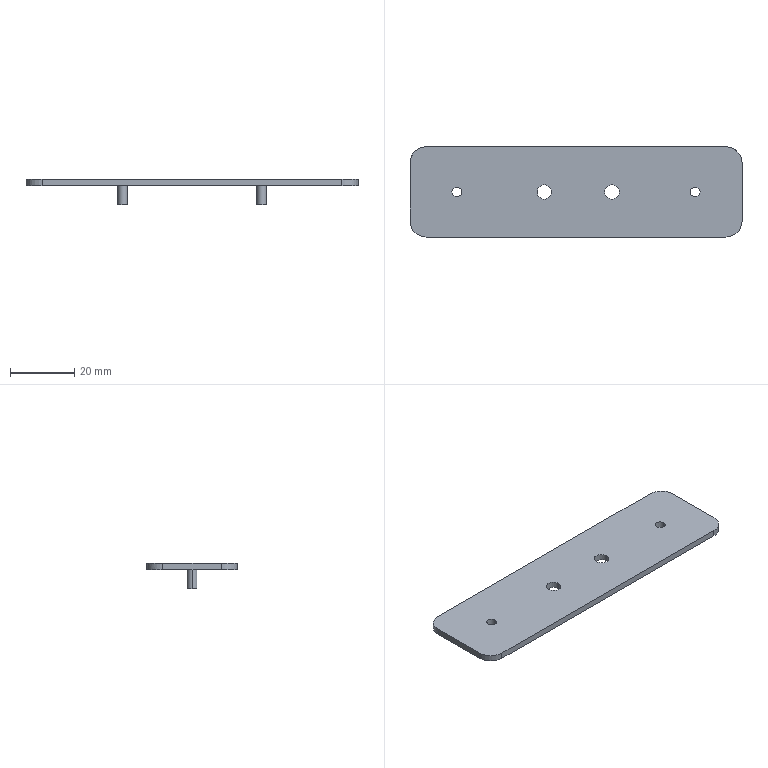Part | NX | features BREP 1 | 1 solid | 24 faces | box 103 x 28 x 8 mm | volume 5718 mm3 | cylinder 16 | plane 8 | commonest cylinder face diameters 3 x8 4.5 x4 10 x4
STEP:
#1=CARTESIAN_POINT('',(-357.75,160.5,217.465));
#2=VERTEX_POINT('',#1);
#3=CARTESIAN_POINT('',(-357.75,160.5,219.465));
#4=VERTEX_POINT('',#3);
#5=CARTESIAN_POINT('',(-357.75,160.5,217.465));
#6=DIRECTION('',(0.,0.,1.));
#7=VECTOR('',#6,1000.);
#8=LINE('',#5,#7);
#9=EDGE_CURVE('',#2,#4,#8,.T.);
#10=ORIENTED_EDGE('',*,*,#9,.T.);
#11=CARTESIAN_POINT('',(-353.25,160.5,219.465));
#12=VERTEX_POINT('',#11);
#13=CARTESIAN_POINT('',(-355.5,160.5,219.465));
#14=DIRECTION('',(0.,0.,-1.));
#15=DIRECTION('',(1.,0.,0.));
#16=AXIS2_PLACEMENT_3D('',#13,#14,#15);
#17=CIRCLE('',#16,2.25);
#18=EDGE_CURVE('',#12,#4,#17,.T.);
#19=ORIENTED_EDGE('',*,*,#18,.F.);
#20=CARTESIAN_POINT('',(-353.25,160.5,217.465));
#21=VERTEX_POINT('',#20);
#22=CARTESIAN_POINT('',(-353.25,160.5,217.465));
#23=DIRECTION('',(0.,0.,-1.));
#24=VECTOR('',#23,1000.);
#25=LINE('',#22,#24);
#26=EDGE_CURVE('',#12,#21,#25,.T.);
#27=ORIENTED_EDGE('',*,*,#26,.T.);
#28=CARTESIAN_POINT('',(-355.5,160.5,217.465));
#29=DIRECTION('',(0.,0.,1.));
#30=DIRECTION('',(1.,0.,0.));
#31=AXIS2_PLACEMENT_3D('',#28,#29,#30);
#32=CIRCLE('',#31,2.25);
#33=EDGE_CURVE('',#2,#21,#32,.T.);
#34=ORIENTED_EDGE('',*,*,#33,.F.);
#35=EDGE_LOOP('',(#10,#19,#27,#34));
#36=FACE_BOUND('',#35,.T.);
#37=CARTESIAN_POINT('',(-355.5,160.5,217.465));
#38=DIRECTION('',(0.,0.,1.));
#39=DIRECTION('',(1.,0.,0.));
#40=AXIS2_PLACEMENT_3D('',#37,#38,#39);
#41=CYLINDRICAL_SURFACE('',#40,2.25);
#42=ADVANCED_FACE('',(#36),#41,.F.);
#43=ORIENTED_EDGE('',*,*,#26,.F.);
#44=CARTESIAN_POINT('',(-355.5,160.5,219.465));
#45=DIRECTION('',(0.,0.,-1.));
#46=DIRECTION('',(1.,0.,0.));
#47=AXIS2_PLACEMENT_3D('',#44,#45,#46);
#48=CIRCLE('',#47,2.25);
#49=EDGE_CURVE('',#4,#12,#48,.T.);
#50=ORIENTED_EDGE('',*,*,#49,.F.);
#51=ORIENTED_EDGE('',*,*,#9,.F.);
#52=CARTESIAN_POINT('',(-355.5,160.5,217.465));
#53=DIRECTION('',(0.,0.,1.));
#54=DIRECTION('',(1.,0.,0.));
#55=AXIS2_PLACEMENT_3D('',#52,#53,#54);
#56=CIRCLE('',#55,2.25);
#57=EDGE_CURVE('',#21,#2,#56,.T.);
#58=ORIENTED_EDGE('',*,*,#57,.F.);
#59=EDGE_LOOP('',(#43,#50,#51,#58));
#60=FACE_BOUND('',#59,.T.);
#61=CARTESIAN_POINT('',(-355.5,160.5,217.465));
#62=DIRECTION('',(0.,0.,1.));
#63=DIRECTION('',(-1.,0.,0.));
#64=AXIS2_PLACEMENT_3D('',#61,#62,#63);
#65=CYLINDRICAL_SURFACE('',#64,2.25);
#66=ADVANCED_FACE('',(#60),#65,.F.);
#67=CARTESIAN_POINT('',(-294.175,169.5,219.465));
#68=VERTEX_POINT('',#67);
#69=CARTESIAN_POINT('',(-294.175,151.5,219.465));
#70=VERTEX_POINT('',#69);
#71=CARTESIAN_POINT('',(-294.175,160.5,219.465));
#72=DIRECTION('',(0.,-1.,0.));
#73=VECTOR('',#72,1000.);
#74=LINE('',#71,#73);
#75=EDGE_CURVE('',#68,#70,#74,.T.);
#76=ORIENTED_EDGE('',*,*,#75,.F.);
#77=CARTESIAN_POINT('',(-299.175,174.5,219.465));
#78=VERTEX_POINT('',#77);
#79=CARTESIAN_POINT('',(-299.175,174.5,219.465));
#80=CARTESIAN_POINT('',(-298.627,174.5,219.465));
#81=CARTESIAN_POINT('',(-298.08,174.425,219.465));
#82=CARTESIAN_POINT('',(-297.546,174.275,219.465));
#83=CARTESIAN_POINT('',(-296.532,173.833,219.465));
#84=CARTESIAN_POINT('',(-295.675,173.134,219.465));
#85=CARTESIAN_POINT('',(-295.297,172.728,219.465));
#86=CARTESIAN_POINT('',(-294.705,171.882,219.465));
#87=CARTESIAN_POINT('',(-294.344,170.917,219.465));
#88=CARTESIAN_POINT('',(-294.231,170.451,219.465));
#89=CARTESIAN_POINT('',(-294.175,169.975,219.465));
#90=CARTESIAN_POINT('',(-294.175,169.5,219.465));
#91=B_SPLINE_CURVE_WITH_KNOTS('',5,(#79,#80,#81,#82,#83,#84,#85,#86,#87,#88,#89,#90),.UNSPECIFIED.,.F.,.F.,(6,3,3,6),(0.,0.3487,0.6974,1.),.UNSPECIFIED.);
#92=EDGE_CURVE('',#78,#68,#91,.T.);
#93=ORIENTED_EDGE('',*,*,#92,.F.);
#94=CARTESIAN_POINT('',(-392.175,174.5,219.465));
#95=VERTEX_POINT('',#94);
#96=CARTESIAN_POINT('',(-345.675,174.5,219.465));
#97=DIRECTION('',(-1.,0.,0.));
#98=VECTOR('',#97,1000.);
#99=LINE('',#96,#98);
#100=EDGE_CURVE('',#78,#95,#99,.T.);
#101=ORIENTED_EDGE('',*,*,#100,.T.);
#102=CARTESIAN_POINT('',(-397.175,169.5,219.465));
#103=VERTEX_POINT('',#102);
#104=CARTESIAN_POINT('',(-397.175,169.5,219.465));
#105=CARTESIAN_POINT('',(-397.175,170.048,219.465));
#106=CARTESIAN_POINT('',(-397.1,170.595,219.465));
#107=CARTESIAN_POINT('',(-396.95,171.129,219.465));
#108=CARTESIAN_POINT('',(-396.508,172.143,219.465));
#109=CARTESIAN_POINT('',(-395.809,173.,219.465));
#110=CARTESIAN_POINT('',(-395.403,173.378,219.465));
#111=CARTESIAN_POINT('',(-394.557,173.97,219.465));
#112=CARTESIAN_POINT('',(-393.592,174.331,219.465));
#113=CARTESIAN_POINT('',(-393.126,174.444,219.465));
#114=CARTESIAN_POINT('',(-392.65,174.5,219.465));
#115=CARTESIAN_POINT('',(-392.175,174.5,219.465));
#116=B_SPLINE_CURVE_WITH_KNOTS('',5,(#104,#105,#106,#107,#108,#109,#110,#111,#112,#113,#114,#115),.UNSPECIFIED.,.F.,.F.,(6,3,3,6),(0.,0.3487,0.6974,1.),.UNSPECIFIED.);
#117=EDGE_CURVE('',#103,#95,#116,.T.);
#118=ORIENTED_EDGE('',*,*,#117,.F.);
#119=CARTESIAN_POINT('',(-397.175,151.5,219.465));
#120=VERTEX_POINT('',#119);
#121=CARTESIAN_POINT('',(-397.175,160.5,219.465));
#122=DIRECTION('',(0.,-1.,0.));
#123=VECTOR('',#122,1000.);
#124=LINE('',#121,#123);
#125=EDGE_CURVE('',#103,#120,#124,.T.);
#126=ORIENTED_EDGE('',*,*,#125,.T.);
#127=CARTESIAN_POINT('',(-392.175,146.5,219.465));
#128=VERTEX_POINT('',#127);
#129=CARTESIAN_POINT('',(-392.175,151.5,219.465));
#130=DIRECTION('',(0.,0.,-1.));
#131=DIRECTION('',(1.,0.,0.));
#132=AXIS2_PLACEMENT_3D('',#129,#130,#131);
#133=CIRCLE('',#132,5.);
#134=EDGE_CURVE('',#128,#120,#133,.T.);
#135=ORIENTED_EDGE('',*,*,#134,.F.);
#136=CARTESIAN_POINT('',(-299.175,146.5,219.465));
#137=VERTEX_POINT('',#136);
#138=CARTESIAN_POINT('',(-345.675,146.5,219.465));
#139=DIRECTION('',(-1.,0.,0.));
#140=VECTOR('',#139,1000.);
#141=LINE('',#138,#140);
#142=EDGE_CURVE('',#137,#128,#141,.T.);
#143=ORIENTED_EDGE('',*,*,#142,.F.);
#144=CARTESIAN_POINT('',(-299.175,151.5,219.465));
#145=DIRECTION('',(0.,0.,-1.));
#146=DIRECTION('',(1.,0.,0.));
#147=AXIS2_PLACEMENT_3D('',#144,#145,#146);
#148=CIRCLE('',#147,5.);
#149=EDGE_CURVE('',#70,#137,#148,.T.);
#150=ORIENTED_EDGE('',*,*,#149,.F.);
#151=EDGE_LOOP('',(#76,#93,#101,#118,#126,#135,#143,#150));
#152=FACE_BOUND('',#151,.T.);
#153=CARTESIAN_POINT('',(-332.25,160.5,219.465));
#154=VERTEX_POINT('',#153);
#155=CARTESIAN_POINT('',(-336.75,160.5,219.465));
#156=VERTEX_POINT('',#155);
#157=CARTESIAN_POINT('',(-334.5,160.5,219.465));
#158=DIRECTION('',(0.,0.,-1.));
#159=DIRECTION('',(1.,0.,0.));
#160=AXIS2_PLACEMENT_3D('',#157,#158,#159);
#161=CIRCLE('',#160,2.25);
#162=EDGE_CURVE('',#154,#156,#161,.T.);
#163=ORIENTED_EDGE('',*,*,#162,.T.);
#164=CARTESIAN_POINT('',(-334.5,160.5,219.465));
#165=DIRECTION('',(0.,0.,-1.));
#166=DIRECTION('',(1.,0.,0.));
#167=AXIS2_PLACEMENT_3D('',#164,#165,#166);
#168=CIRCLE('',#167,2.25);
#169=EDGE_CURVE('',#156,#154,#168,.T.);
#170=ORIENTED_EDGE('',*,*,#169,.T.);
#171=EDGE_LOOP('',(#163,#170));
#172=FACE_BOUND('',#171,.T.);
#173=CARTESIAN_POINT('',(-307.175,160.5,219.465));
#174=VERTEX_POINT('',#173);
#175=CARTESIAN_POINT('',(-310.175,160.5,219.465));
#176=VERTEX_POINT('',#175);
#177=CARTESIAN_POINT('',(-308.675,160.5,219.465));
#178=DIRECTION('',(0.,0.,-1.));
#179=DIRECTION('',(1.,0.,0.));
#180=AXIS2_PLACEMENT_3D('',#177,#178,#179);
#181=CIRCLE('',#180,1.5);
#182=EDGE_CURVE('',#174,#176,#181,.T.);
#183=ORIENTED_EDGE('',*,*,#182,.T.);
#184=CARTESIAN_POINT('',(-308.675,160.5,219.465));
#185=DIRECTION('',(0.,0.,-1.));
#186=DIRECTION('',(1.,0.,0.));
#187=AXIS2_PLACEMENT_3D('',#184,#185,#186);
#188=CIRCLE('',#187,1.5);
#189=EDGE_CURVE('',#176,#174,#188,.T.);
#190=ORIENTED_EDGE('',*,*,#189,.T.);
#191=EDGE_LOOP('',(#183,#190));
#192=FACE_BOUND('',#191,.T.);
#193=ORIENTED_EDGE('',*,*,#49,.T.);
#194=ORIENTED_EDGE('',*,*,#18,.T.);
#195=EDGE_LOOP('',(#193,#194));
#196=FACE_BOUND('',#195,.T.);
#197=CARTESIAN_POINT('',(-384.175,160.5,219.465));
#198=VERTEX_POINT('',#197);
#199=CARTESIAN_POINT('',(-381.175,160.5,219.465));
#200=VERTEX_POINT('',#199);
#201=CARTESIAN_POINT('',(-382.675,160.5,219.465));
#202=DIRECTION('',(0.,0.,-1.));
#203=DIRECTION('',(1.,0.,0.));
#204=AXIS2_PLACEMENT_3D('',#201,#202,#203);
#205=CIRCLE('',#204,1.5);
#206=EDGE_CURVE('',#198,#200,#205,.T.);
#207=ORIENTED_EDGE('',*,*,#206,.T.);
#208=CARTESIAN_POINT('',(-382.675,160.5,219.465));
#209=DIRECTION('',(0.,0.,-1.));
#210=DIRECTION('',(1.,0.,0.));
#211=AXIS2_PLACEMENT_3D('',#208,#209,#210);
#212=CIRCLE('',#211,1.5);
#213=EDGE_CURVE('',#200,#198,#212,.T.);
#214=ORIENTED_EDGE('',*,*,#213,.T.);
#215=EDGE_LOOP('',(#207,#214));
#216=FACE_BOUND('',#215,.T.);
#217=CARTESIAN_POINT('',(74.,-121.964,219.465));
#218=DIRECTION('',(0.,0.,1.));
#219=DIRECTION('',(1.,0.,0.));
#220=AXIS2_PLACEMENT_3D('',#217,#218,#219);
#221=PLANE('',#220);
#222=ADVANCED_FACE('',(#152,#172,#192,#196,#216),#221,.T.);
#223=CARTESIAN_POINT('',(-299.175,146.5,217.465));
#224=VERTEX_POINT('',#223);
#225=CARTESIAN_POINT('',(-294.175,151.5,217.465));
#226=VERTEX_POINT('',#225);
#227=CARTESIAN_POINT('',(-299.175,151.5,217.465));
#228=DIRECTION('',(0.,0.,1.));
#229=DIRECTION('',(1.,0.,0.));
#230=AXIS2_PLACEMENT_3D('',#227,#228,#229);
#231=CIRCLE('',#230,5.);
#232=EDGE_CURVE('',#224,#226,#231,.T.);
#233=ORIENTED_EDGE('',*,*,#232,.F.);
#234=CARTESIAN_POINT('',(-392.175,146.5,217.465));
#235=VERTEX_POINT('',#234);
#236=CARTESIAN_POINT('',(-345.675,146.5,217.465));
#237=DIRECTION('',(-1.,0.,0.));
#238=VECTOR('',#237,1000.);
#239=LINE('',#236,#238);
#240=EDGE_CURVE('',#224,#235,#239,.T.);
#241=ORIENTED_EDGE('',*,*,#240,.T.);
#242=CARTESIAN_POINT('',(-397.175,151.5,217.465));
#243=VERTEX_POINT('',#242);
#244=CARTESIAN_POINT('',(-392.175,151.5,217.465));
#245=DIRECTION('',(0.,0.,1.));
#246=DIRECTION('',(1.,0.,0.));
#247=AXIS2_PLACEMENT_3D('',#244,#245,#246);
#248=CIRCLE('',#247,5.);
#249=EDGE_CURVE('',#243,#235,#248,.T.);
#250=ORIENTED_EDGE('',*,*,#249,.F.);
#251=CARTESIAN_POINT('',(-397.175,169.5,217.465));
#252=VERTEX_POINT('',#251);
#253=CARTESIAN_POINT('',(-397.175,160.5,217.465));
#254=DIRECTION('',(0.,-1.,0.));
#255=VECTOR('',#254,1000.);
#256=LINE('',#253,#255);
#257=EDGE_CURVE('',#252,#243,#256,.T.);
#258=ORIENTED_EDGE('',*,*,#257,.F.);
#259=CARTESIAN_POINT('',(-392.175,174.5,217.465));
#260=VERTEX_POINT('',#259);
#261=CARTESIAN_POINT('',(-392.175,174.5,217.465));
#262=CARTESIAN_POINT('',(-392.65,174.5,217.465));
#263=CARTESIAN_POINT('',(-393.126,174.444,217.465));
#264=CARTESIAN_POINT('',(-393.592,174.331,217.465));
#265=CARTESIAN_POINT('',(-394.557,173.97,217.465));
#266=CARTESIAN_POINT('',(-395.403,173.378,217.465));
#267=CARTESIAN_POINT('',(-395.809,173.,217.465));
#268=CARTESIAN_POINT('',(-396.508,172.143,217.465));
#269=CARTESIAN_POINT('',(-396.95,171.129,217.465));
#270=CARTESIAN_POINT('',(-397.1,170.595,217.465));
#271=CARTESIAN_POINT('',(-397.175,170.048,217.465));
#272=CARTESIAN_POINT('',(-397.175,169.5,217.465));
#273=B_SPLINE_CURVE_WITH_KNOTS('',5,(#261,#262,#263,#264,#265,#266,#267,#268,#269,#270,#271,#272),.UNSPECIFIED.,.F.,.F.,(6,3,3,6),(0.,0.3026,0.6513,1.),.UNSPECIFIED.);
#274=EDGE_CURVE('',#260,#252,#273,.T.);
#275=ORIENTED_EDGE('',*,*,#274,.F.);
#276=CARTESIAN_POINT('',(-299.175,174.5,217.465));
#277=VERTEX_POINT('',#276);
#278=CARTESIAN_POINT('',(-345.675,174.5,217.465));
#279=DIRECTION('',(-1.,0.,0.));
#280=VECTOR('',#279,1000.);
#281=LINE('',#278,#280);
#282=EDGE_CURVE('',#277,#260,#281,.T.);
#283=ORIENTED_EDGE('',*,*,#282,.F.);
#284=CARTESIAN_POINT('',(-294.175,169.5,217.465));
#285=VERTEX_POINT('',#284);
#286=CARTESIAN_POINT('',(-294.175,169.5,217.465));
#287=CARTESIAN_POINT('',(-294.175,169.975,217.465));
#288=CARTESIAN_POINT('',(-294.231,170.451,217.465));
#289=CARTESIAN_POINT('',(-294.344,170.917,217.465));
#290=CARTESIAN_POINT('',(-294.705,171.882,217.465));
#291=CARTESIAN_POINT('',(-295.297,172.728,217.465));
#292=CARTESIAN_POINT('',(-295.675,173.134,217.465));
#293=CARTESIAN_POINT('',(-296.532,173.833,217.465));
#294=CARTESIAN_POINT('',(-297.546,174.275,217.465));
#295=CARTESIAN_POINT('',(-298.08,174.425,217.465));
#296=CARTESIAN_POINT('',(-298.627,174.5,217.465));
#297=CARTESIAN_POINT('',(-299.175,174.5,217.465));
#298=B_SPLINE_CURVE_WITH_KNOTS('',5,(#286,#287,#288,#289,#290,#291,#292,#293,#294,#295,#296,#297),.UNSPECIFIED.,.F.,.F.,(6,3,3,6),(0.,0.3026,0.6513,1.),.UNSPECIFIED.);
#299=EDGE_CURVE('',#285,#277,#298,.T.);
#300=ORIENTED_EDGE('',*,*,#299,.F.);
#301=CARTESIAN_POINT('',(-294.175,160.5,217.465));
#302=DIRECTION('',(0.,-1.,0.));
#303=VECTOR('',#302,1000.);
#304=LINE('',#301,#303);
#305=EDGE_CURVE('',#285,#226,#304,.T.);
#306=ORIENTED_EDGE('',*,*,#305,.T.);
#307=EDGE_LOOP('',(#233,#241,#250,#258,#275,#283,#300,#306));
#308=FACE_BOUND('',#307,.T.);
#309=CARTESIAN_POINT('',(-322.675,160.5,217.465));
#310=VERTEX_POINT('',#309);
#311=CARTESIAN_POINT('',(-325.675,160.5,217.465));
#312=VERTEX_POINT('',#311);
#313=CARTESIAN_POINT('',(-324.175,160.5,217.465));
#314=DIRECTION('',(0.,0.,1.));
#315=DIRECTION('',(1.,0.,0.));
#316=AXIS2_PLACEMENT_3D('',#313,#314,#315);
#317=CIRCLE('',#316,1.5);
#318=EDGE_CURVE('',#310,#312,#317,.T.);
#319=ORIENTED_EDGE('',*,*,#318,.T.);
#320=CARTESIAN_POINT('',(-324.175,160.5,217.465));
#321=DIRECTION('',(0.,0.,1.));
#322=DIRECTION('',(1.,0.,0.));
#323=AXIS2_PLACEMENT_3D('',#320,#321,#322);
#324=CIRCLE('',#323,1.5);
#325=EDGE_CURVE('',#312,#310,#324,.T.);
#326=ORIENTED_EDGE('',*,*,#325,.T.);
#327=EDGE_LOOP('',(#319,#326));
#328=FACE_BOUND('',#327,.T.);
#329=CARTESIAN_POINT('',(-365.675,160.5,217.465));
#330=VERTEX_POINT('',#329);
#331=CARTESIAN_POINT('',(-368.675,160.5,217.465));
#332=VERTEX_POINT('',#331);
#333=CARTESIAN_POINT('',(-367.175,160.5,217.465));
#334=DIRECTION('',(0.,0.,1.));
#335=DIRECTION('',(1.,0.,0.));
#336=AXIS2_PLACEMENT_3D('',#333,#334,#335);
#337=CIRCLE('',#336,1.5);
#338=EDGE_CURVE('',#330,#332,#337,.T.);
#339=ORIENTED_EDGE('',*,*,#338,.T.);
#340=CARTESIAN_POINT('',(-367.175,160.5,217.465));
#341=DIRECTION('',(0.,0.,1.));
#342=DIRECTION('',(1.,0.,0.));
#343=AXIS2_PLACEMENT_3D('',#340,#341,#342);
#344=CIRCLE('',#343,1.5);
#345=EDGE_CURVE('',#332,#330,#344,.T.);
#346=ORIENTED_EDGE('',*,*,#345,.T.);
#347=EDGE_LOOP('',(#339,#346));
#348=FACE_BOUND('',#347,.T.);
#349=ORIENTED_EDGE('',*,*,#57,.T.);
#350=ORIENTED_EDGE('',*,*,#33,.T.);
#351=EDGE_LOOP('',(#349,#350));
#352=FACE_BOUND('',#351,.T.);
#353=CARTESIAN_POINT('',(-332.25,160.5,217.465));
#354=VERTEX_POINT('',#353);
#355=CARTESIAN_POINT('',(-336.75,160.5,217.465));
#356=VERTEX_POINT('',#355);
#357=CARTESIAN_POINT('',(-334.5,160.5,217.465));
#358=DIRECTION('',(0.,0.,1.));
#359=DIRECTION('',(1.,0.,0.));
#360=AXIS2_PLACEMENT_3D('',#357,#358,#359);
#361=CIRCLE('',#360,2.25);
#362=EDGE_CURVE('',#354,#356,#361,.T.);
#363=ORIENTED_EDGE('',*,*,#362,.T.);
#364=CARTESIAN_POINT('',(-334.5,160.5,217.465));
#365=DIRECTION('',(0.,0.,1.));
#366=DIRECTION('',(1.,0.,0.));
#367=AXIS2_PLACEMENT_3D('',#364,#365,#366);
#368=CIRCLE('',#367,2.25);
#369=EDGE_CURVE('',#356,#354,#368,.T.);
#370=ORIENTED_EDGE('',*,*,#369,.T.);
#371=EDGE_LOOP('',(#363,#370));
#372=FACE_BOUND('',#371,.T.);
#373=CARTESIAN_POINT('',(-381.175,160.5,217.465));
#374=VERTEX_POINT('',#373);
#375=CARTESIAN_POINT('',(-384.175,160.5,217.465));
#376=VERTEX_POINT('',#375);
#377=CARTESIAN_POINT('',(-382.675,160.5,217.465));
#378=DIRECTION('',(0.,0.,1.));
#379=DIRECTION('',(1.,0.,0.));
#380=AXIS2_PLACEMENT_3D('',#377,#378,#379);
#381=CIRCLE('',#380,1.5);
#382=EDGE_CURVE('',#374,#376,#381,.T.);
#383=ORIENTED_EDGE('',*,*,#382,.T.);
#384=CARTESIAN_POINT('',(-382.675,160.5,217.465));
#385=DIRECTION('',(0.,0.,1.));
#386=DIRECTION('',(1.,0.,0.));
#387=AXIS2_PLACEMENT_3D('',#384,#385,#386);
#388=CIRCLE('',#387,1.5);
#389=EDGE_CURVE('',#376,#374,#388,.T.);
#390=ORIENTED_EDGE('',*,*,#389,.T.);
#391=EDGE_LOOP('',(#383,#390));
#392=FACE_BOUND('',#391,.T.);
#393=CARTESIAN_POINT('',(-307.175,160.5,217.465));
#394=VERTEX_POINT('',#393);
#395=CARTESIAN_POINT('',(-310.175,160.5,217.465));
#396=VERTEX_POINT('',#395);
#397=CARTESIAN_POINT('',(-308.675,160.5,217.465));
#398=DIRECTION('',(0.,0.,1.));
#399=DIRECTION('',(1.,0.,0.));
#400=AXIS2_PLACEMENT_3D('',#397,#398,#399);
#401=CIRCLE('',#400,1.5);
#402=EDGE_CURVE('',#394,#396,#401,.T.);
#403=ORIENTED_EDGE('',*,*,#402,.T.);
#404=CARTESIAN_POINT('',(-308.675,160.5,217.465));
#405=DIRECTION('',(0.,0.,1.));
#406=DIRECTION('',(1.,0.,0.));
#407=AXIS2_PLACEMENT_3D('',#404,#405,#406);
#408=CIRCLE('',#407,1.5);
#409=EDGE_CURVE('',#396,#394,#408,.T.);
#410=ORIENTED_EDGE('',*,*,#409,.T.);
#411=EDGE_LOOP('',(#403,#410));
#412=FACE_BOUND('',#411,.T.);
#413=CARTESIAN_POINT('',(74.,-121.964,217.465));
#414=DIRECTION('',(0.,0.,1.));
#415=DIRECTION('',(1.,0.,0.));
#416=AXIS2_PLACEMENT_3D('',#413,#414,#415);
#417=PLANE('',#416);
#418=ADVANCED_FACE('',(#308,#328,#348,#352,#372,#392,#412),#417,.F.);
#419=ORIENTED_EDGE('',*,*,#305,.F.);
#420=CARTESIAN_POINT('',(-294.175,169.5,218.465));
#421=DIRECTION('',(0.,-0.000000001,-1.));
#422=VECTOR('',#421,1000.);
#423=LINE('',#420,#422);
#424=EDGE_CURVE('',#68,#285,#423,.T.);
#425=ORIENTED_EDGE('',*,*,#424,.F.);
#426=ORIENTED_EDGE('',*,*,#75,.T.);
#427=CARTESIAN_POINT('',(-294.175,151.5,218.465));
#428=DIRECTION('',(0.,0.,1.));
#429=VECTOR('',#428,1000.);
#430=LINE('',#427,#429);
#431=EDGE_CURVE('',#226,#70,#430,.T.);
#432=ORIENTED_EDGE('',*,*,#431,.F.);
#433=EDGE_LOOP('',(#419,#425,#426,#432));
#434=FACE_BOUND('',#433,.T.);
#435=CARTESIAN_POINT('',(-294.175,146.5,217.465));
#436=DIRECTION('',(1.,0.,0.));
#437=DIRECTION('',(0.,1.,0.));
#438=AXIS2_PLACEMENT_3D('',#435,#436,#437);
#439=PLANE('',#438);
#440=ADVANCED_FACE('',(#434),#439,.T.);
#441=ORIENTED_EDGE('',*,*,#299,.T.);
#442=CARTESIAN_POINT('',(-299.175,174.5,218.465));
#443=DIRECTION('',(0.,0.,-1.));
#444=VECTOR('',#443,1000.);
#445=LINE('',#442,#444);
#446=EDGE_CURVE('',#78,#277,#445,.T.);
#447=ORIENTED_EDGE('',*,*,#446,.F.);
#448=ORIENTED_EDGE('',*,*,#92,.T.);
#449=ORIENTED_EDGE('',*,*,#424,.T.);
#450=EDGE_LOOP('',(#441,#447,#448,#449));
#451=FACE_BOUND('',#450,.T.);
#452=CARTESIAN_POINT('',(-299.175,169.5,218.465));
#453=DIRECTION('',(0.,0.,-1.));
#454=DIRECTION('',(0.,-1.,0.));
#455=AXIS2_PLACEMENT_3D('',#452,#453,#454);
#456=CYLINDRICAL_SURFACE('',#455,5.);
#457=ADVANCED_FACE('',(#451),#456,.T.);
#458=ORIENTED_EDGE('',*,*,#282,.T.);
#459=CARTESIAN_POINT('',(-392.175,174.5,218.465));
#460=DIRECTION('',(0.,0.,-1.));
#461=VECTOR('',#460,1000.);
#462=LINE('',#459,#461);
#463=EDGE_CURVE('',#95,#260,#462,.T.);
#464=ORIENTED_EDGE('',*,*,#463,.F.);
#465=ORIENTED_EDGE('',*,*,#100,.F.);
#466=ORIENTED_EDGE('',*,*,#446,.T.);
#467=EDGE_LOOP('',(#458,#464,#465,#466));
#468=FACE_BOUND('',#467,.T.);
#469=CARTESIAN_POINT('',(-294.125,174.5,217.465));
#470=DIRECTION('',(0.,1.,0.));
#471=DIRECTION('',(1.,0.,0.));
#472=AXIS2_PLACEMENT_3D('',#469,#470,#471);
#473=PLANE('',#472);
#474=ADVANCED_FACE('',(#468),#473,.T.);
#475=ORIENTED_EDGE('',*,*,#274,.T.);
#476=CARTESIAN_POINT('',(-397.175,169.5,218.465));
#477=DIRECTION('',(0.,0.,-1.));
#478=VECTOR('',#477,1000.);
#479=LINE('',#476,#478);
#480=EDGE_CURVE('',#103,#252,#479,.T.);
#481=ORIENTED_EDGE('',*,*,#480,.F.);
#482=ORIENTED_EDGE('',*,*,#117,.T.);
#483=ORIENTED_EDGE('',*,*,#463,.T.);
#484=EDGE_LOOP('',(#475,#481,#482,#483));
#485=FACE_BOUND('',#484,.T.);
#486=CARTESIAN_POINT('',(-392.175,169.5,218.465));
#487=DIRECTION('',(0.,0.,-1.));
#488=DIRECTION('',(1.,0.,0.));
#489=AXIS2_PLACEMENT_3D('',#486,#487,#488);
#490=CYLINDRICAL_SURFACE('',#489,5.);
#491=ADVANCED_FACE('',(#485),#490,.T.);
#492=ORIENTED_EDGE('',*,*,#125,.F.);
#493=ORIENTED_EDGE('',*,*,#480,.T.);
#494=ORIENTED_EDGE('',*,*,#257,.T.);
#495=CARTESIAN_POINT('',(-397.175,151.5,218.465));
#496=DIRECTION('',(0.,0.,1.));
#497=VECTOR('',#496,1000.);
#498=LINE('',#495,#497);
#499=EDGE_CURVE('',#243,#120,#498,.T.);
#500=ORIENTED_EDGE('',*,*,#499,.T.);
#501=EDGE_LOOP('',(#492,#493,#494,#500));
#502=FACE_BOUND('',#501,.T.);
#503=CARTESIAN_POINT('',(-397.175,174.5,217.465));
#504=DIRECTION('',(-1.,0.,0.));
#505=DIRECTION('',(0.,0.,1.));
#506=AXIS2_PLACEMENT_3D('',#503,#504,#505);
#507=PLANE('',#506);
#508=ADVANCED_FACE('',(#502),#507,.T.);
#509=ORIENTED_EDGE('',*,*,#134,.T.);
#510=ORIENTED_EDGE('',*,*,#499,.F.);
#511=ORIENTED_EDGE('',*,*,#249,.T.);
#512=CARTESIAN_POINT('',(-392.175,146.5,218.465));
#513=DIRECTION('',(0.,0.,1.));
#514=VECTOR('',#513,1000.);
#515=LINE('',#512,#514);
#516=EDGE_CURVE('',#235,#128,#515,.T.);
#517=ORIENTED_EDGE('',*,*,#516,.T.);
#518=EDGE_LOOP('',(#509,#510,#511,#517));
#519=FACE_BOUND('',#518,.T.);
#520=CARTESIAN_POINT('',(-392.175,151.5,218.465));
#521=DIRECTION('',(0.,0.,1.));
#522=DIRECTION('',(1.,0.,0.));
#523=AXIS2_PLACEMENT_3D('',#520,#521,#522);
#524=CYLINDRICAL_SURFACE('',#523,5.);
#525=ADVANCED_FACE('',(#519),#524,.T.);
#526=ORIENTED_EDGE('',*,*,#142,.T.);
#527=ORIENTED_EDGE('',*,*,#516,.F.);
#528=ORIENTED_EDGE('',*,*,#240,.F.);
#529=CARTESIAN_POINT('',(-299.175,146.5,218.465));
#530=DIRECTION('',(0.,0.,1.));
#531=VECTOR('',#530,1000.);
#532=LINE('',#529,#531);
#533=EDGE_CURVE('',#224,#137,#532,.T.);
#534=ORIENTED_EDGE('',*,*,#533,.T.);
#535=EDGE_LOOP('',(#526,#527,#528,#534));
#536=FACE_BOUND('',#535,.T.);
#537=CARTESIAN_POINT('',(-397.225,146.5,217.465));
#538=DIRECTION('',(0.,-1.,0.));
#539=DIRECTION('',(0.,0.,-1.));
#540=AXIS2_PLACEMENT_3D('',#537,#538,#539);
#541=PLANE('',#540);
#542=ADVANCED_FACE('',(#536),#541,.T.);
#543=ORIENTED_EDGE('',*,*,#149,.T.);
#544=ORIENTED_EDGE('',*,*,#533,.F.);
#545=ORIENTED_EDGE('',*,*,#232,.T.);
#546=ORIENTED_EDGE('',*,*,#431,.T.);
#547=EDGE_LOOP('',(#543,#544,#545,#546));
#548=FACE_BOUND('',#547,.T.);
#549=CARTESIAN_POINT('',(-299.175,151.5,218.465));
#550=DIRECTION('',(0.,0.,1.));
#551=DIRECTION('',(0.,1.,0.));
#552=AXIS2_PLACEMENT_3D('',#549,#550,#551);
#553=CYLINDRICAL_SURFACE('',#552,5.);
#554=ADVANCED_FACE('',(#548),#553,.T.);
#555=CARTESIAN_POINT('',(-336.75,160.5,217.465));
#556=DIRECTION('',(0.,0.,1.));
#557=VECTOR('',#556,1000.);
#558=LINE('',#555,#557);
#559=EDGE_CURVE('',#356,#156,#558,.T.);
#560=ORIENTED_EDGE('',*,*,#559,.T.);
#561=ORIENTED_EDGE('',*,*,#162,.F.);
#562=CARTESIAN_POINT('',(-332.25,160.5,217.465));
#563=DIRECTION('',(0.,0.,-1.));
#564=VECTOR('',#563,1000.);
#565=LINE('',#562,#564);
#566=EDGE_CURVE('',#154,#354,#565,.T.);
#567=ORIENTED_EDGE('',*,*,#566,.T.);
#568=ORIENTED_EDGE('',*,*,#369,.F.);
#569=EDGE_LOOP('',(#560,#561,#567,#568));
#570=FACE_BOUND('',#569,.T.);
#571=CARTESIAN_POINT('',(-334.5,160.5,217.465));
#572=DIRECTION('',(0.,0.,1.));
#573=DIRECTION('',(1.,0.,0.));
#574=AXIS2_PLACEMENT_3D('',#571,#572,#573);
#575=CYLINDRICAL_SURFACE('',#574,2.25);
#576=ADVANCED_FACE('',(#570),#575,.F.);
#577=ORIENTED_EDGE('',*,*,#566,.F.);
#578=ORIENTED_EDGE('',*,*,#169,.F.);
#579=ORIENTED_EDGE('',*,*,#559,.F.);
#580=ORIENTED_EDGE('',*,*,#362,.F.);
#581=EDGE_LOOP('',(#577,#578,#579,#580));
#582=FACE_BOUND('',#581,.T.);
#583=CARTESIAN_POINT('',(-334.5,160.5,217.465));
#584=DIRECTION('',(0.,0.,1.));
#585=DIRECTION('',(-1.,0.,0.));
#586=AXIS2_PLACEMENT_3D('',#583,#584,#585);
#587=CYLINDRICAL_SURFACE('',#586,2.25);
#588=ADVANCED_FACE('',(#582),#587,.F.);
#589=CARTESIAN_POINT('',(-310.175,160.5,217.465));
#590=DIRECTION('',(0.,0.,1.));
#591=VECTOR('',#590,1000.);
#592=LINE('',#589,#591);
#593=EDGE_CURVE('',#396,#176,#592,.T.);
#594=ORIENTED_EDGE('',*,*,#593,.T.);
#595=ORIENTED_EDGE('',*,*,#182,.F.);
#596=CARTESIAN_POINT('',(-307.175,160.5,217.465));
#597=DIRECTION('',(0.,0.,-1.));
#598=VECTOR('',#597,1000.);
#599=LINE('',#596,#598);
#600=EDGE_CURVE('',#174,#394,#599,.T.);
#601=ORIENTED_EDGE('',*,*,#600,.T.);
#602=ORIENTED_EDGE('',*,*,#409,.F.);
#603=EDGE_LOOP('',(#594,#595,#601,#602));
#604=FACE_BOUND('',#603,.T.);
#605=CARTESIAN_POINT('',(-308.675,160.5,217.465));
#606=DIRECTION('',(0.,0.,1.));
#607=DIRECTION('',(1.,0.,0.));
#608=AXIS2_PLACEMENT_3D('',#605,#606,#607);
#609=CYLINDRICAL_SURFACE('',#608,1.5);
#610=ADVANCED_FACE('',(#604),#609,.F.);
#611=ORIENTED_EDGE('',*,*,#600,.F.);
#612=ORIENTED_EDGE('',*,*,#189,.F.);
#613=ORIENTED_EDGE('',*,*,#593,.F.);
#614=ORIENTED_EDGE('',*,*,#402,.F.);
#615=EDGE_LOOP('',(#611,#612,#613,#614));
#616=FACE_BOUND('',#615,.T.);
#617=CARTESIAN_POINT('',(-308.675,160.5,217.465));
#618=DIRECTION('',(0.,0.,1.));
#619=DIRECTION('',(-1.,0.,0.));
#620=AXIS2_PLACEMENT_3D('',#617,#618,#619);
#621=CYLINDRICAL_SURFACE('',#620,1.5);
#622=ADVANCED_FACE('',(#616),#621,.F.);
#623=CARTESIAN_POINT('',(-381.175,160.5,217.465));
#624=DIRECTION('',(0.,0.,-1.));
#625=VECTOR('',#624,1000.);
#626=LINE('',#623,#625);
#627=EDGE_CURVE('',#200,#374,#626,.T.);
#628=ORIENTED_EDGE('',*,*,#627,.F.);
#629=ORIENTED_EDGE('',*,*,#206,.F.);
#630=CARTESIAN_POINT('',(-384.175,160.5,217.465));
#631=DIRECTION('',(0.,0.,1.));
#632=VECTOR('',#631,1000.);
#633=LINE('',#630,#632);
#634=EDGE_CURVE('',#376,#198,#633,.T.);
#635=ORIENTED_EDGE('',*,*,#634,.F.);
#636=ORIENTED_EDGE('',*,*,#382,.F.);
#637=EDGE_LOOP('',(#628,#629,#635,#636));
#638=FACE_BOUND('',#637,.T.);
#639=CARTESIAN_POINT('',(-382.675,160.5,217.465));
#640=DIRECTION('',(0.,0.,1.));
#641=DIRECTION('',(-1.,0.,0.));
#642=AXIS2_PLACEMENT_3D('',#639,#640,#641);
#643=CYLINDRICAL_SURFACE('',#642,1.5);
#644=ADVANCED_FACE('',(#638),#643,.F.);
#645=ORIENTED_EDGE('',*,*,#634,.T.);
#646=ORIENTED_EDGE('',*,*,#213,.F.);
#647=ORIENTED_EDGE('',*,*,#627,.T.);
#648=ORIENTED_EDGE('',*,*,#389,.F.);
#649=EDGE_LOOP('',(#645,#646,#647,#648));
#650=FACE_BOUND('',#649,.T.);
#651=CARTESIAN_POINT('',(-382.675,160.5,217.465));
#652=DIRECTION('',(0.,0.,1.));
#653=DIRECTION('',(1.,0.,0.));
#654=AXIS2_PLACEMENT_3D('',#651,#652,#653);
#655=CYLINDRICAL_SURFACE('',#654,1.5);
#656=ADVANCED_FACE('',(#650),#655,.F.);
#657=CARTESIAN_POINT('',(-322.675,160.5,211.465));
#658=VERTEX_POINT('',#657);
#659=CARTESIAN_POINT('',(-325.675,160.5,211.465));
#660=VERTEX_POINT('',#659);
#661=CARTESIAN_POINT('',(-324.175,160.5,211.465));
#662=DIRECTION('',(0.,0.,1.));
#663=DIRECTION('',(1.,0.,0.));
#664=AXIS2_PLACEMENT_3D('',#661,#662,#663);
#665=CIRCLE('',#664,1.5);
#666=EDGE_CURVE('',#658,#660,#665,.T.);
#667=ORIENTED_EDGE('',*,*,#666,.F.);
#668=CARTESIAN_POINT('',(-324.175,160.5,211.465));
#669=DIRECTION('',(0.,0.,1.));
#670=DIRECTION('',(1.,0.,0.));
#671=AXIS2_PLACEMENT_3D('',#668,#669,#670);
#672=CIRCLE('',#671,1.5);
#673=EDGE_CURVE('',#660,#658,#672,.T.);
#674=ORIENTED_EDGE('',*,*,#673,.F.);
#675=EDGE_LOOP('',(#667,#674));
#676=FACE_BOUND('',#675,.T.);
#677=CARTESIAN_POINT('',(0.,0.,211.465));
#678=DIRECTION('',(0.,0.,1.));
#679=DIRECTION('',(-1.,0.,0.));
#680=AXIS2_PLACEMENT_3D('',#677,#678,#679);
#681=PLANE('',#680);
#682=ADVANCED_FACE('',(#676),#681,.F.);
#683=CARTESIAN_POINT('',(-365.675,160.5,211.465));
#684=VERTEX_POINT('',#683);
#685=CARTESIAN_POINT('',(-368.675,160.5,211.465));
#686=VERTEX_POINT('',#685);
#687=CARTESIAN_POINT('',(-367.175,160.5,211.465));
#688=DIRECTION('',(0.,0.,1.));
#689=DIRECTION('',(1.,0.,0.));
#690=AXIS2_PLACEMENT_3D('',#687,#688,#689);
#691=CIRCLE('',#690,1.5);
#692=EDGE_CURVE('',#684,#686,#691,.T.);
#693=ORIENTED_EDGE('',*,*,#692,.F.);
#694=CARTESIAN_POINT('',(-367.175,160.5,211.465));
#695=DIRECTION('',(0.,0.,1.));
#696=DIRECTION('',(1.,0.,0.));
#697=AXIS2_PLACEMENT_3D('',#694,#695,#696);
#698=CIRCLE('',#697,1.5);
#699=EDGE_CURVE('',#686,#684,#698,.T.);
#700=ORIENTED_EDGE('',*,*,#699,.F.);
#701=EDGE_LOOP('',(#693,#700));
#702=FACE_BOUND('',#701,.T.);
#703=CARTESIAN_POINT('',(0.,0.,211.465));
#704=DIRECTION('',(0.,0.,1.));
#705=DIRECTION('',(-1.,0.,0.));
#706=AXIS2_PLACEMENT_3D('',#703,#704,#705);
#707=PLANE('',#706);
#708=ADVANCED_FACE('',(#702),#707,.F.);
#709=CARTESIAN_POINT('',(-365.675,160.5,216.465));
#710=DIRECTION('',(0.,0.,-1.));
#711=VECTOR('',#710,1000.);
#712=LINE('',#709,#711);
#713=EDGE_CURVE('',#330,#684,#712,.T.);
#714=ORIENTED_EDGE('',*,*,#713,.F.);
#715=ORIENTED_EDGE('',*,*,#345,.F.);
#716=CARTESIAN_POINT('',(-368.675,160.5,216.465));
#717=DIRECTION('',(0.,0.,-1.));
#718=VECTOR('',#717,1000.);
#719=LINE('',#716,#718);
#720=EDGE_CURVE('',#332,#686,#719,.T.);
#721=ORIENTED_EDGE('',*,*,#720,.T.);
#722=ORIENTED_EDGE('',*,*,#699,.T.);
#723=EDGE_LOOP('',(#714,#715,#721,#722));
#724=FACE_BOUND('',#723,.T.);
#725=CARTESIAN_POINT('',(-367.175,160.5,216.465));
#726=DIRECTION('',(0.,0.,1.));
#727=DIRECTION('',(1.,0.,0.));
#728=AXIS2_PLACEMENT_3D('',#725,#726,#727);
#729=CYLINDRICAL_SURFACE('',#728,1.5);
#730=ADVANCED_FACE('',(#724),#729,.T.);
#731=ORIENTED_EDGE('',*,*,#713,.T.);
#732=ORIENTED_EDGE('',*,*,#692,.T.);
#733=ORIENTED_EDGE('',*,*,#720,.F.);
#734=ORIENTED_EDGE('',*,*,#338,.F.);
#735=EDGE_LOOP('',(#731,#732,#733,#734));
#736=FACE_BOUND('',#735,.T.);
#737=CARTESIAN_POINT('',(-367.175,160.5,216.465));
#738=DIRECTION('',(0.,0.,1.));
#739=DIRECTION('',(-1.,0.,0.));
#740=AXIS2_PLACEMENT_3D('',#737,#738,#739);
#741=CYLINDRICAL_SURFACE('',#740,1.5);
#742=ADVANCED_FACE('',(#736),#741,.T.);
#743=CARTESIAN_POINT('',(-322.675,160.5,216.465));
#744=DIRECTION('',(0.,0.,-1.));
#745=VECTOR('',#744,1000.);
#746=LINE('',#743,#745);
#747=EDGE_CURVE('',#310,#658,#746,.T.);
#748=ORIENTED_EDGE('',*,*,#747,.F.);
#749=ORIENTED_EDGE('',*,*,#325,.F.);
#750=CARTESIAN_POINT('',(-325.675,160.5,216.465));
#751=DIRECTION('',(0.,0.,-1.));
#752=VECTOR('',#751,1000.);
#753=LINE('',#750,#752);
#754=EDGE_CURVE('',#312,#660,#753,.T.);
#755=ORIENTED_EDGE('',*,*,#754,.T.);
#756=ORIENTED_EDGE('',*,*,#673,.T.);
#757=EDGE_LOOP('',(#748,#749,#755,#756));
#758=FACE_BOUND('',#757,.T.);
#759=CARTESIAN_POINT('',(-324.175,160.5,216.465));
#760=DIRECTION('',(0.,0.,1.));
#761=DIRECTION('',(1.,0.,0.));
#762=AXIS2_PLACEMENT_3D('',#759,#760,#761);
#763=CYLINDRICAL_SURFACE('',#762,1.5);
#764=ADVANCED_FACE('',(#758),#763,.T.);
#765=ORIENTED_EDGE('',*,*,#747,.T.);
#766=ORIENTED_EDGE('',*,*,#666,.T.);
#767=ORIENTED_EDGE('',*,*,#754,.F.);
#768=ORIENTED_EDGE('',*,*,#318,.F.);
#769=EDGE_LOOP('',(#765,#766,#767,#768));
#770=FACE_BOUND('',#769,.T.);
#771=CARTESIAN_POINT('',(-324.175,160.5,216.465));
#772=DIRECTION('',(0.,0.,1.));
#773=DIRECTION('',(-1.,0.,0.));
#774=AXIS2_PLACEMENT_3D('',#771,#772,#773);
#775=CYLINDRICAL_SURFACE('',#774,1.5);
#776=ADVANCED_FACE('',(#770),#775,.T.);
#777=CLOSED_SHELL('',(#42,#66,#222,#418,#440,#457,#474,#491,#508,#525,#542,#554,#576,#588,#610,#622,#644,#656,#682,#708,#730,#742,#764,#776));
#778=MANIFOLD_SOLID_BREP('',#777);
#779=(LENGTH_UNIT()NAMED_UNIT(*)SI_UNIT(.MILLI.,.METRE.));
#780=UNCERTAINTY_MEASURE_WITH_UNIT(LENGTH_MEASURE(0.00001),#779,'','');
#781=(NAMED_UNIT(*)PLANE_ANGLE_UNIT()SI_UNIT($,.RADIAN.));
#782=(NAMED_UNIT(*)SI_UNIT($,.STERADIAN.)SOLID_ANGLE_UNIT());
#783=(GEOMETRIC_REPRESENTATION_CONTEXT(3)GLOBAL_UNCERTAINTY_ASSIGNED_CONTEXT((#780))GLOBAL_UNIT_ASSIGNED_CONTEXT((#779,#781,#782))REPRESENTATION_CONTEXT('',''));
#784=ADVANCED_BREP_SHAPE_REPRESENTATION('',(#778),#783);